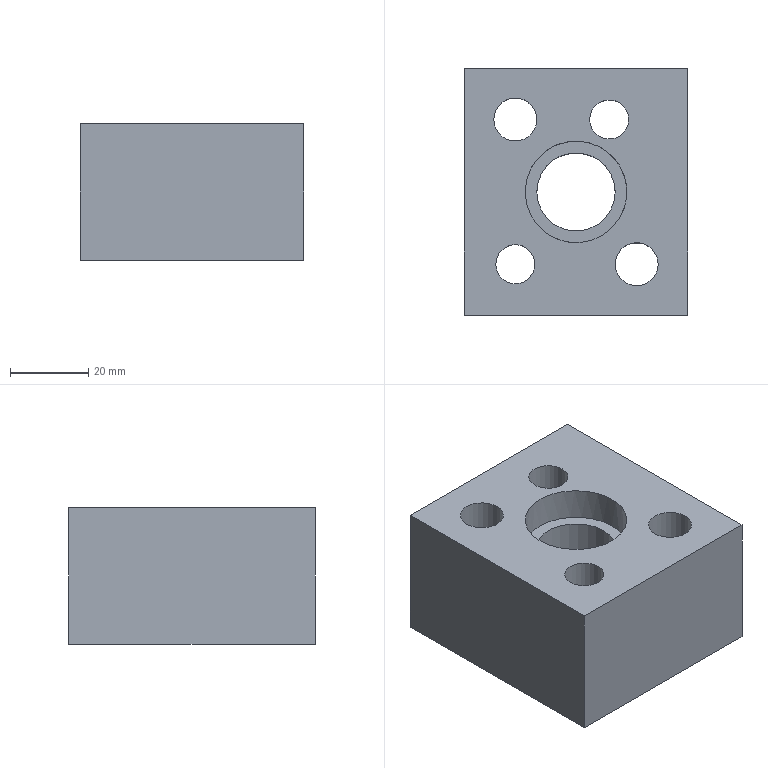Part | NX | features solid 2 | 1 solid | 21 faces | box 57 x 63 x 35 mm | volume 95221 mm3 | plane 11 | cylinder 10 | commonest cylinder face diameters 10 x2 10.5 x2 11 x2 17 x2 20 x1 26 x1
STEP:
#1=CARTESIAN_POINT('',(138.75,121.5,58.));
#2=VERTEX_POINT('',#1);
#3=CARTESIAN_POINT('',(133.5,121.5,58.));
#4=DIRECTION('',(0.,0.,1.));
#5=DIRECTION('',(1.,0.,0.));
#6=AXIS2_PLACEMENT_3D('',#3,#4,#5);
#7=CIRCLE('',#6,5.25);
#8=EDGE_CURVE('',#2,#2,#7,.F.);
#9=ORIENTED_EDGE('',*,*,#8,.F.);
#10=EDGE_LOOP('',(#9));
#11=FACE_BOUND('',#10,.T.);
#12=CARTESIAN_POINT('',(128.25,121.5,43.));
#13=VERTEX_POINT('',#12);
#14=CARTESIAN_POINT('',(133.5,121.5,43.));
#15=DIRECTION('',(0.,0.,-1.));
#16=DIRECTION('',(-1.,0.,0.));
#17=AXIS2_PLACEMENT_3D('',#14,#15,#16);
#18=CIRCLE('',#17,5.25);
#19=EDGE_CURVE('',#13,#13,#18,.F.);
#20=ORIENTED_EDGE('',*,*,#19,.F.);
#21=EDGE_LOOP('',(#20));
#22=FACE_BOUND('',#21,.T.);
#23=CARTESIAN_POINT('',(133.5,121.5,43.));
#24=DIRECTION('',(0.,0.,1.));
#25=DIRECTION('',(1.,0.,0.));
#26=AXIS2_PLACEMENT_3D('',#23,#24,#25);
#27=CYLINDRICAL_SURFACE('',#26,5.25);
#28=ADVANCED_FACE('',(#11,#22),#27,.F.);
#29=CARTESIAN_POINT('',(138.5,121.5,58.));
#30=VERTEX_POINT('',#29);
#31=CARTESIAN_POINT('',(133.5,121.5,58.));
#32=DIRECTION('',(0.,0.,1.));
#33=DIRECTION('',(1.,0.,0.));
#34=AXIS2_PLACEMENT_3D('',#31,#32,#33);
#35=CIRCLE('',#34,5.);
#36=EDGE_CURVE('',#30,#30,#35,.F.);
#37=ORIENTED_EDGE('',*,*,#36,.F.);
#38=EDGE_LOOP('',(#37));
#39=FACE_BOUND('',#38,.T.);
#40=ORIENTED_EDGE('',*,*,#8,.T.);
#41=EDGE_LOOP('',(#40));
#42=FACE_BOUND('',#41,.T.);
#43=CARTESIAN_POINT('',(155.126,171.473,58.));
#44=DIRECTION('',(0.,0.,1.));
#45=DIRECTION('',(-1.,0.,0.));
#46=AXIS2_PLACEMENT_3D('',#43,#44,#45);
#47=PLANE('',#46);
#48=ADVANCED_FACE('',(#39,#42),#47,.F.);
#49=CARTESIAN_POINT('',(128.5,121.5,78.));
#50=VERTEX_POINT('',#49);
#51=CARTESIAN_POINT('',(133.5,121.5,78.));
#52=DIRECTION('',(0.,0.,-1.));
#53=DIRECTION('',(-1.,0.,0.));
#54=AXIS2_PLACEMENT_3D('',#51,#52,#53);
#55=CIRCLE('',#54,5.);
#56=EDGE_CURVE('',#50,#50,#55,.T.);
#57=ORIENTED_EDGE('',*,*,#56,.F.);
#58=EDGE_LOOP('',(#57));
#59=FACE_BOUND('',#58,.T.);
#60=ORIENTED_EDGE('',*,*,#36,.T.);
#61=EDGE_LOOP('',(#60));
#62=FACE_BOUND('',#61,.T.);
#63=CARTESIAN_POINT('',(133.5,121.5,78.));
#64=DIRECTION('',(0.,0.,1.));
#65=DIRECTION('',(1.,0.,0.));
#66=AXIS2_PLACEMENT_3D('',#63,#64,#65);
#67=CYLINDRICAL_SURFACE('',#66,5.);
#68=ADVANCED_FACE('',(#59,#62),#67,.F.);
#69=CARTESIAN_POINT('',(159.,121.5,78.));
#70=VERTEX_POINT('',#69);
#71=CARTESIAN_POINT('',(164.5,121.5,78.));
#72=DIRECTION('',(0.,0.,1.));
#73=DIRECTION('',(-1.,0.,0.));
#74=AXIS2_PLACEMENT_3D('',#71,#72,#73);
#75=CIRCLE('',#74,5.5);
#76=EDGE_CURVE('',#70,#70,#75,.F.);
#77=ORIENTED_EDGE('',*,*,#76,.F.);
#78=EDGE_LOOP('',(#77));
#79=FACE_BOUND('',#78,.T.);
#80=CARTESIAN_POINT('',(159.,121.5,63.));
#81=VERTEX_POINT('',#80);
#82=CARTESIAN_POINT('',(164.5,121.5,63.));
#83=DIRECTION('',(0.,0.,1.));
#84=DIRECTION('',(-1.,0.,0.));
#85=AXIS2_PLACEMENT_3D('',#82,#83,#84);
#86=CIRCLE('',#85,5.5);
#87=EDGE_CURVE('',#81,#81,#86,.F.);
#88=ORIENTED_EDGE('',*,*,#87,.T.);
#89=EDGE_LOOP('',(#88));
#90=FACE_BOUND('',#89,.T.);
#91=CARTESIAN_POINT('',(164.5,121.5,78.));
#92=DIRECTION('',(0.,0.,1.));
#93=DIRECTION('',(-1.,0.,0.));
#94=AXIS2_PLACEMENT_3D('',#91,#92,#93);
#95=CYLINDRICAL_SURFACE('',#94,5.5);
#96=ADVANCED_FACE('',(#79,#90),#95,.F.);
#97=ORIENTED_EDGE('',*,*,#87,.F.);
#98=EDGE_LOOP('',(#97));
#99=FACE_BOUND('',#98,.T.);
#100=CARTESIAN_POINT('',(156.,121.5,63.));
#101=VERTEX_POINT('',#100);
#102=CARTESIAN_POINT('',(164.5,121.5,63.));
#103=DIRECTION('',(0.,0.,1.));
#104=DIRECTION('',(-1.,0.,0.));
#105=AXIS2_PLACEMENT_3D('',#102,#103,#104);
#106=CIRCLE('',#105,8.5);
#107=EDGE_CURVE('',#101,#101,#106,.F.);
#108=ORIENTED_EDGE('',*,*,#107,.T.);
#109=EDGE_LOOP('',(#108));
#110=FACE_BOUND('',#109,.T.);
#111=CARTESIAN_POINT('',(162.126,122.527,63.));
#112=DIRECTION('',(0.,0.,1.));
#113=DIRECTION('',(-1.,0.,0.));
#114=AXIS2_PLACEMENT_3D('',#111,#112,#113);
#115=PLANE('',#114);
#116=ADVANCED_FACE('',(#99,#110),#115,.F.);
#117=ORIENTED_EDGE('',*,*,#107,.F.);
#118=EDGE_LOOP('',(#117));
#119=FACE_BOUND('',#118,.T.);
#120=CARTESIAN_POINT('',(156.,121.5,43.));
#121=VERTEX_POINT('',#120);
#122=CARTESIAN_POINT('',(164.5,121.5,43.));
#123=DIRECTION('',(0.,0.,1.));
#124=DIRECTION('',(-1.,0.,0.));
#125=AXIS2_PLACEMENT_3D('',#122,#123,#124);
#126=CIRCLE('',#125,8.5);
#127=EDGE_CURVE('',#121,#121,#126,.T.);
#128=ORIENTED_EDGE('',*,*,#127,.F.);
#129=EDGE_LOOP('',(#128));
#130=FACE_BOUND('',#129,.T.);
#131=CARTESIAN_POINT('',(164.5,121.5,43.));
#132=DIRECTION('',(0.,0.,1.));
#133=DIRECTION('',(-1.,0.,0.));
#134=AXIS2_PLACEMENT_3D('',#131,#132,#133);
#135=CYLINDRICAL_SURFACE('',#134,8.5);
#136=ADVANCED_FACE('',(#119,#130),#135,.F.);
#137=CARTESIAN_POINT('',(139.,158.5,63.));
#138=VERTEX_POINT('',#137);
#139=CARTESIAN_POINT('',(133.5,158.5,63.));
#140=DIRECTION('',(0.,0.,1.));
#141=DIRECTION('',(1.,0.,0.));
#142=AXIS2_PLACEMENT_3D('',#139,#140,#141);
#143=CIRCLE('',#142,5.5);
#144=EDGE_CURVE('',#138,#138,#143,.F.);
#145=ORIENTED_EDGE('',*,*,#144,.F.);
#146=EDGE_LOOP('',(#145));
#147=FACE_BOUND('',#146,.T.);
#148=CARTESIAN_POINT('',(142.,158.5,63.));
#149=VERTEX_POINT('',#148);
#150=CARTESIAN_POINT('',(133.5,158.5,63.));
#151=DIRECTION('',(0.,0.,1.));
#152=DIRECTION('',(1.,0.,0.));
#153=AXIS2_PLACEMENT_3D('',#150,#151,#152);
#154=CIRCLE('',#153,8.5);
#155=EDGE_CURVE('',#149,#149,#154,.F.);
#156=ORIENTED_EDGE('',*,*,#155,.T.);
#157=EDGE_LOOP('',(#156));
#158=FACE_BOUND('',#157,.T.);
#159=CARTESIAN_POINT('',(135.874,157.473,63.));
#160=DIRECTION('',(0.,0.,1.));
#161=DIRECTION('',(1.,0.,0.));
#162=AXIS2_PLACEMENT_3D('',#159,#160,#161);
#163=PLANE('',#162);
#164=ADVANCED_FACE('',(#147,#158),#163,.F.);
#165=CARTESIAN_POINT('',(162.5,158.5,58.));
#166=VERTEX_POINT('',#165);
#167=CARTESIAN_POINT('',(157.5,158.5,58.));
#168=DIRECTION('',(0.,0.,1.));
#169=DIRECTION('',(1.,0.,0.));
#170=AXIS2_PLACEMENT_3D('',#167,#168,#169);
#171=CIRCLE('',#170,5.);
#172=EDGE_CURVE('',#166,#166,#171,.F.);
#173=ORIENTED_EDGE('',*,*,#172,.F.);
#174=EDGE_LOOP('',(#173));
#175=FACE_BOUND('',#174,.T.);
#176=CARTESIAN_POINT('',(162.75,158.5,58.));
#177=VERTEX_POINT('',#176);
#178=CARTESIAN_POINT('',(157.5,158.5,58.));
#179=DIRECTION('',(0.,0.,1.));
#180=DIRECTION('',(1.,0.,0.));
#181=AXIS2_PLACEMENT_3D('',#178,#179,#180);
#182=CIRCLE('',#181,5.25);
#183=EDGE_CURVE('',#177,#177,#182,.F.);
#184=ORIENTED_EDGE('',*,*,#183,.T.);
#185=EDGE_LOOP('',(#184));
#186=FACE_BOUND('',#185,.T.);
#187=CARTESIAN_POINT('',(155.126,157.473,58.));
#188=DIRECTION('',(0.,0.,1.));
#189=DIRECTION('',(-1.,0.,0.));
#190=AXIS2_PLACEMENT_3D('',#187,#188,#189);
#191=PLANE('',#190);
#192=ADVANCED_FACE('',(#175,#186),#191,.F.);
#193=CARTESIAN_POINT('',(120.5,171.5,78.));
#194=VERTEX_POINT('',#193);
#195=CARTESIAN_POINT('',(120.5,171.5,43.));
#196=VERTEX_POINT('',#195);
#197=CARTESIAN_POINT('',(120.5,171.5,78.));
#198=DIRECTION('',(0.,0.,-1.));
#199=VECTOR('',#198,1000.);
#200=LINE('',#197,#199);
#201=EDGE_CURVE('',#194,#196,#200,.T.);
#202=ORIENTED_EDGE('',*,*,#201,.F.);
#203=CARTESIAN_POINT('',(177.5,171.5,78.));
#204=VERTEX_POINT('',#203);
#205=CARTESIAN_POINT('',(149.,171.5,78.));
#206=DIRECTION('',(1.,0.,0.));
#207=VECTOR('',#206,1000.);
#208=LINE('',#205,#207);
#209=EDGE_CURVE('',#204,#194,#208,.F.);
#210=ORIENTED_EDGE('',*,*,#209,.F.);
#211=CARTESIAN_POINT('',(177.5,171.5,43.));
#212=VERTEX_POINT('',#211);
#213=CARTESIAN_POINT('',(177.5,171.5,78.));
#214=DIRECTION('',(0.,0.,-1.));
#215=VECTOR('',#214,1000.);
#216=LINE('',#213,#215);
#217=EDGE_CURVE('',#204,#212,#216,.T.);
#218=ORIENTED_EDGE('',*,*,#217,.T.);
#219=CARTESIAN_POINT('',(149.,171.5,43.));
#220=DIRECTION('',(1.,0.,0.));
#221=VECTOR('',#220,1000.);
#222=LINE('',#219,#221);
#223=EDGE_CURVE('',#212,#196,#222,.F.);
#224=ORIENTED_EDGE('',*,*,#223,.T.);
#225=EDGE_LOOP('',(#202,#210,#218,#224));
#226=FACE_BOUND('',#225,.T.);
#227=CARTESIAN_POINT('',(149.,171.5,78.));
#228=DIRECTION('',(0.,-1.,0.));
#229=DIRECTION('',(-1.,0.,0.));
#230=AXIS2_PLACEMENT_3D('',#227,#228,#229);
#231=PLANE('',#230);
#232=ADVANCED_FACE('',(#226),#231,.F.);
#233=CARTESIAN_POINT('',(120.5,108.5,78.));
#234=VERTEX_POINT('',#233);
#235=CARTESIAN_POINT('',(120.5,108.5,43.));
#236=VERTEX_POINT('',#235);
#237=CARTESIAN_POINT('',(120.5,108.5,78.));
#238=DIRECTION('',(0.,0.,-1.));
#239=VECTOR('',#238,1000.);
#240=LINE('',#237,#239);
#241=EDGE_CURVE('',#234,#236,#240,.T.);
#242=ORIENTED_EDGE('',*,*,#241,.F.);
#243=CARTESIAN_POINT('',(120.5,140.,78.));
#244=DIRECTION('',(0.,1.,0.));
#245=VECTOR('',#244,1000.);
#246=LINE('',#243,#245);
#247=EDGE_CURVE('',#194,#234,#246,.F.);
#248=ORIENTED_EDGE('',*,*,#247,.F.);
#249=ORIENTED_EDGE('',*,*,#201,.T.);
#250=CARTESIAN_POINT('',(120.5,140.,43.));
#251=DIRECTION('',(0.,1.,0.));
#252=VECTOR('',#251,1000.);
#253=LINE('',#250,#252);
#254=EDGE_CURVE('',#196,#236,#253,.F.);
#255=ORIENTED_EDGE('',*,*,#254,.T.);
#256=EDGE_LOOP('',(#242,#248,#249,#255));
#257=FACE_BOUND('',#256,.T.);
#258=CARTESIAN_POINT('',(120.5,140.,78.));
#259=DIRECTION('',(1.,0.,0.));
#260=DIRECTION('',(0.,-1.,0.));
#261=AXIS2_PLACEMENT_3D('',#258,#259,#260);
#262=PLANE('',#261);
#263=ADVANCED_FACE('',(#257),#262,.F.);
#264=CARTESIAN_POINT('',(177.5,108.5,78.));
#265=VERTEX_POINT('',#264);
#266=CARTESIAN_POINT('',(149.,108.5,78.));
#267=DIRECTION('',(-1.,0.,0.));
#268=VECTOR('',#267,1000.);
#269=LINE('',#266,#268);
#270=EDGE_CURVE('',#234,#265,#269,.F.);
#271=ORIENTED_EDGE('',*,*,#270,.F.);
#272=ORIENTED_EDGE('',*,*,#241,.T.);
#273=CARTESIAN_POINT('',(177.5,108.5,43.));
#274=VERTEX_POINT('',#273);
#275=CARTESIAN_POINT('',(149.,108.5,43.));
#276=DIRECTION('',(-1.,0.,0.));
#277=VECTOR('',#276,1000.);
#278=LINE('',#275,#277);
#279=EDGE_CURVE('',#236,#274,#278,.F.);
#280=ORIENTED_EDGE('',*,*,#279,.T.);
#281=CARTESIAN_POINT('',(177.5,108.5,78.));
#282=DIRECTION('',(0.,0.,-1.));
#283=VECTOR('',#282,1000.);
#284=LINE('',#281,#283);
#285=EDGE_CURVE('',#265,#274,#284,.T.);
#286=ORIENTED_EDGE('',*,*,#285,.F.);
#287=EDGE_LOOP('',(#271,#272,#280,#286));
#288=FACE_BOUND('',#287,.T.);
#289=CARTESIAN_POINT('',(149.,108.5,78.));
#290=DIRECTION('',(0.,1.,0.));
#291=DIRECTION('',(1.,0.,0.));
#292=AXIS2_PLACEMENT_3D('',#289,#290,#291);
#293=PLANE('',#292);
#294=ADVANCED_FACE('',(#288),#293,.F.);
#295=ORIENTED_EDGE('',*,*,#217,.F.);
#296=CARTESIAN_POINT('',(177.5,140.,78.));
#297=DIRECTION('',(0.,-1.,0.));
#298=VECTOR('',#297,1000.);
#299=LINE('',#296,#298);
#300=EDGE_CURVE('',#265,#204,#299,.F.);
#301=ORIENTED_EDGE('',*,*,#300,.F.);
#302=ORIENTED_EDGE('',*,*,#285,.T.);
#303=CARTESIAN_POINT('',(177.5,140.,43.));
#304=DIRECTION('',(0.,-1.,0.));
#305=VECTOR('',#304,1000.);
#306=LINE('',#303,#305);
#307=EDGE_CURVE('',#274,#212,#306,.F.);
#308=ORIENTED_EDGE('',*,*,#307,.T.);
#309=EDGE_LOOP('',(#295,#301,#302,#308));
#310=FACE_BOUND('',#309,.T.);
#311=CARTESIAN_POINT('',(177.5,140.,78.));
#312=DIRECTION('',(-1.,0.,0.));
#313=DIRECTION('',(0.,1.,0.));
#314=AXIS2_PLACEMENT_3D('',#311,#312,#313);
#315=PLANE('',#314);
#316=ADVANCED_FACE('',(#310),#315,.F.);
#317=ORIENTED_EDGE('',*,*,#155,.F.);
#318=EDGE_LOOP('',(#317));
#319=FACE_BOUND('',#318,.T.);
#320=CARTESIAN_POINT('',(142.,158.5,43.));
#321=VERTEX_POINT('',#320);
#322=CARTESIAN_POINT('',(133.5,158.5,43.));
#323=DIRECTION('',(0.,0.,1.));
#324=DIRECTION('',(1.,0.,0.));
#325=AXIS2_PLACEMENT_3D('',#322,#323,#324);
#326=CIRCLE('',#325,8.5);
#327=EDGE_CURVE('',#321,#321,#326,.T.);
#328=ORIENTED_EDGE('',*,*,#327,.F.);
#329=EDGE_LOOP('',(#328));
#330=FACE_BOUND('',#329,.T.);
#331=CARTESIAN_POINT('',(133.5,158.5,43.));
#332=DIRECTION('',(0.,0.,1.));
#333=DIRECTION('',(1.,0.,0.));
#334=AXIS2_PLACEMENT_3D('',#331,#332,#333);
#335=CYLINDRICAL_SURFACE('',#334,8.5);
#336=ADVANCED_FACE('',(#319,#330),#335,.F.);
#337=ORIENTED_EDGE('',*,*,#183,.F.);
#338=EDGE_LOOP('',(#337));
#339=FACE_BOUND('',#338,.T.);
#340=CARTESIAN_POINT('',(152.25,158.5,43.));
#341=VERTEX_POINT('',#340);
#342=CARTESIAN_POINT('',(157.5,158.5,43.));
#343=DIRECTION('',(0.,0.,-1.));
#344=DIRECTION('',(-1.,0.,0.));
#345=AXIS2_PLACEMENT_3D('',#342,#343,#344);
#346=CIRCLE('',#345,5.25);
#347=EDGE_CURVE('',#341,#341,#346,.F.);
#348=ORIENTED_EDGE('',*,*,#347,.F.);
#349=EDGE_LOOP('',(#348));
#350=FACE_BOUND('',#349,.T.);
#351=CARTESIAN_POINT('',(157.5,158.5,43.));
#352=DIRECTION('',(0.,0.,1.));
#353=DIRECTION('',(-1.,0.,0.));
#354=AXIS2_PLACEMENT_3D('',#351,#352,#353);
#355=CYLINDRICAL_SURFACE('',#354,5.25);
#356=ADVANCED_FACE('',(#339,#350),#355,.F.);
#357=CARTESIAN_POINT('',(139.,140.,43.));
#358=VERTEX_POINT('',#357);
#359=CARTESIAN_POINT('',(149.,140.,43.));
#360=DIRECTION('',(0.,0.,-1.));
#361=DIRECTION('',(-1.,0.,0.));
#362=AXIS2_PLACEMENT_3D('',#359,#360,#361);
#363=CIRCLE('',#362,10.);
#364=EDGE_CURVE('',#358,#358,#363,.F.);
#365=ORIENTED_EDGE('',*,*,#364,.T.);
#366=EDGE_LOOP('',(#365));
#367=FACE_BOUND('',#366,.T.);
#368=ORIENTED_EDGE('',*,*,#19,.T.);
#369=EDGE_LOOP('',(#368));
#370=FACE_BOUND('',#369,.T.);
#371=ORIENTED_EDGE('',*,*,#127,.T.);
#372=EDGE_LOOP('',(#371));
#373=FACE_BOUND('',#372,.T.);
#374=ORIENTED_EDGE('',*,*,#347,.T.);
#375=EDGE_LOOP('',(#374));
#376=FACE_BOUND('',#375,.T.);
#377=ORIENTED_EDGE('',*,*,#327,.T.);
#378=EDGE_LOOP('',(#377));
#379=FACE_BOUND('',#378,.T.);
#380=ORIENTED_EDGE('',*,*,#307,.F.);
#381=ORIENTED_EDGE('',*,*,#279,.F.);
#382=ORIENTED_EDGE('',*,*,#254,.F.);
#383=ORIENTED_EDGE('',*,*,#223,.F.);
#384=EDGE_LOOP('',(#380,#381,#382,#383));
#385=FACE_BOUND('',#384,.T.);
#386=CARTESIAN_POINT('',(149.,140.,43.));
#387=DIRECTION('',(0.,0.,-1.));
#388=DIRECTION('',(-1.,0.,0.));
#389=AXIS2_PLACEMENT_3D('',#386,#387,#388);
#390=PLANE('',#389);
#391=ADVANCED_FACE('',(#367,#370,#373,#376,#379,#385),#390,.T.);
#392=CARTESIAN_POINT('',(139.,158.5,78.));
#393=VERTEX_POINT('',#392);
#394=CARTESIAN_POINT('',(133.5,158.5,78.));
#395=DIRECTION('',(0.,0.,1.));
#396=DIRECTION('',(1.,0.,0.));
#397=AXIS2_PLACEMENT_3D('',#394,#395,#396);
#398=CIRCLE('',#397,5.5);
#399=EDGE_CURVE('',#393,#393,#398,.T.);
#400=ORIENTED_EDGE('',*,*,#399,.T.);
#401=EDGE_LOOP('',(#400));
#402=FACE_BOUND('',#401,.T.);
#403=ORIENTED_EDGE('',*,*,#144,.T.);
#404=EDGE_LOOP('',(#403));
#405=FACE_BOUND('',#404,.T.);
#406=CARTESIAN_POINT('',(133.5,158.5,78.));
#407=DIRECTION('',(0.,0.,1.));
#408=DIRECTION('',(1.,0.,0.));
#409=AXIS2_PLACEMENT_3D('',#406,#407,#408);
#410=CYLINDRICAL_SURFACE('',#409,5.5);
#411=ADVANCED_FACE('',(#402,#405),#410,.F.);
#412=CARTESIAN_POINT('',(152.5,158.5,78.));
#413=VERTEX_POINT('',#412);
#414=CARTESIAN_POINT('',(157.5,158.5,78.));
#415=DIRECTION('',(0.,0.,-1.));
#416=DIRECTION('',(-1.,0.,0.));
#417=AXIS2_PLACEMENT_3D('',#414,#415,#416);
#418=CIRCLE('',#417,5.);
#419=EDGE_CURVE('',#413,#413,#418,.T.);
#420=ORIENTED_EDGE('',*,*,#419,.F.);
#421=EDGE_LOOP('',(#420));
#422=FACE_BOUND('',#421,.T.);
#423=ORIENTED_EDGE('',*,*,#172,.T.);
#424=EDGE_LOOP('',(#423));
#425=FACE_BOUND('',#424,.T.);
#426=CARTESIAN_POINT('',(157.5,158.5,78.));
#427=DIRECTION('',(0.,0.,1.));
#428=DIRECTION('',(-1.,0.,0.));
#429=AXIS2_PLACEMENT_3D('',#426,#427,#428);
#430=CYLINDRICAL_SURFACE('',#429,5.);
#431=ADVANCED_FACE('',(#422,#425),#430,.F.);
#432=CARTESIAN_POINT('',(136.,140.,78.));
#433=VERTEX_POINT('',#432);
#434=CARTESIAN_POINT('',(149.,140.,78.));
#435=DIRECTION('',(0.,0.,-1.));
#436=DIRECTION('',(-1.,0.,0.));
#437=AXIS2_PLACEMENT_3D('',#434,#435,#436);
#438=CIRCLE('',#437,13.);
#439=EDGE_CURVE('',#433,#433,#438,.F.);
#440=ORIENTED_EDGE('',*,*,#439,.F.);
#441=EDGE_LOOP('',(#440));
#442=FACE_BOUND('',#441,.T.);
#443=ORIENTED_EDGE('',*,*,#56,.T.);
#444=EDGE_LOOP('',(#443));
#445=FACE_BOUND('',#444,.T.);
#446=ORIENTED_EDGE('',*,*,#76,.T.);
#447=EDGE_LOOP('',(#446));
#448=FACE_BOUND('',#447,.T.);
#449=ORIENTED_EDGE('',*,*,#419,.T.);
#450=EDGE_LOOP('',(#449));
#451=FACE_BOUND('',#450,.T.);
#452=ORIENTED_EDGE('',*,*,#399,.F.);
#453=EDGE_LOOP('',(#452));
#454=FACE_BOUND('',#453,.T.);
#455=ORIENTED_EDGE('',*,*,#300,.T.);
#456=ORIENTED_EDGE('',*,*,#209,.T.);
#457=ORIENTED_EDGE('',*,*,#247,.T.);
#458=ORIENTED_EDGE('',*,*,#270,.T.);
#459=EDGE_LOOP('',(#455,#456,#457,#458));
#460=FACE_BOUND('',#459,.T.);
#461=CARTESIAN_POINT('',(149.,140.,78.));
#462=DIRECTION('',(0.,0.,-1.));
#463=DIRECTION('',(-1.,0.,0.));
#464=AXIS2_PLACEMENT_3D('',#461,#462,#463);
#465=PLANE('',#464);
#466=ADVANCED_FACE('',(#442,#445,#448,#451,#454,#460),#465,.F.);
#467=ORIENTED_EDGE('',*,*,#364,.F.);
#468=EDGE_LOOP('',(#467));
#469=FACE_BOUND('',#468,.T.);
#470=CARTESIAN_POINT('',(159.,140.,69.7));
#471=VERTEX_POINT('',#470);
#472=CARTESIAN_POINT('',(149.,140.,69.7));
#473=DIRECTION('',(0.,0.,1.));
#474=DIRECTION('',(1.,0.,0.));
#475=AXIS2_PLACEMENT_3D('',#472,#473,#474);
#476=CIRCLE('',#475,10.);
#477=EDGE_CURVE('',#471,#471,#476,.F.);
#478=ORIENTED_EDGE('',*,*,#477,.F.);
#479=EDGE_LOOP('',(#478));
#480=FACE_BOUND('',#479,.T.);
#481=CARTESIAN_POINT('',(149.,140.,82.));
#482=DIRECTION('',(0.,0.,-1.));
#483=DIRECTION('',(-1.,0.,0.));
#484=AXIS2_PLACEMENT_3D('',#481,#482,#483);
#485=CYLINDRICAL_SURFACE('',#484,10.);
#486=ADVANCED_FACE('',(#469,#480),#485,.F.);
#487=ORIENTED_EDGE('',*,*,#439,.T.);
#488=EDGE_LOOP('',(#487));
#489=FACE_BOUND('',#488,.T.);
#490=CARTESIAN_POINT('',(162.,140.,69.7));
#491=VERTEX_POINT('',#490);
#492=CARTESIAN_POINT('',(149.,140.,69.7));
#493=DIRECTION('',(0.,0.,1.));
#494=DIRECTION('',(1.,0.,0.));
#495=AXIS2_PLACEMENT_3D('',#492,#493,#494);
#496=CIRCLE('',#495,13.);
#497=EDGE_CURVE('',#491,#491,#496,.F.);
#498=ORIENTED_EDGE('',*,*,#497,.T.);
#499=EDGE_LOOP('',(#498));
#500=FACE_BOUND('',#499,.T.);
#501=CARTESIAN_POINT('',(149.,140.,82.));
#502=DIRECTION('',(0.,0.,-1.));
#503=DIRECTION('',(-1.,0.,0.));
#504=AXIS2_PLACEMENT_3D('',#501,#502,#503);
#505=CYLINDRICAL_SURFACE('',#504,13.);
#506=ADVANCED_FACE('',(#489,#500),#505,.F.);
#507=ORIENTED_EDGE('',*,*,#477,.T.);
#508=EDGE_LOOP('',(#507));
#509=FACE_BOUND('',#508,.T.);
#510=ORIENTED_EDGE('',*,*,#497,.F.);
#511=EDGE_LOOP('',(#510));
#512=FACE_BOUND('',#511,.T.);
#513=CARTESIAN_POINT('',(149.,140.,69.7));
#514=DIRECTION('',(0.,0.,1.));
#515=DIRECTION('',(1.,0.,0.));
#516=AXIS2_PLACEMENT_3D('',#513,#514,#515);
#517=PLANE('',#516);
#518=ADVANCED_FACE('',(#509,#512),#517,.T.);
#519=CLOSED_SHELL('',(#28,#48,#68,#96,#116,#136,#164,#192,#232,#263,#294,#316,#336,#356,#391,#411,#431,#466,#486,#506,#518));
#520=MANIFOLD_SOLID_BREP('',#519);
#521=(LENGTH_UNIT()NAMED_UNIT(*)SI_UNIT(.MILLI.,.METRE.));
#522=UNCERTAINTY_MEASURE_WITH_UNIT(LENGTH_MEASURE(0.00001),#521,'','');
#523=(NAMED_UNIT(*)PLANE_ANGLE_UNIT()SI_UNIT($,.RADIAN.));
#524=(NAMED_UNIT(*)SI_UNIT($,.STERADIAN.)SOLID_ANGLE_UNIT());
#525=(GEOMETRIC_REPRESENTATION_CONTEXT(3)GLOBAL_UNCERTAINTY_ASSIGNED_CONTEXT((#522))GLOBAL_UNIT_ASSIGNED_CONTEXT((#521,#523,#524))REPRESENTATION_CONTEXT('',''));
#526=ADVANCED_BREP_SHAPE_REPRESENTATION('',(#520),#525);